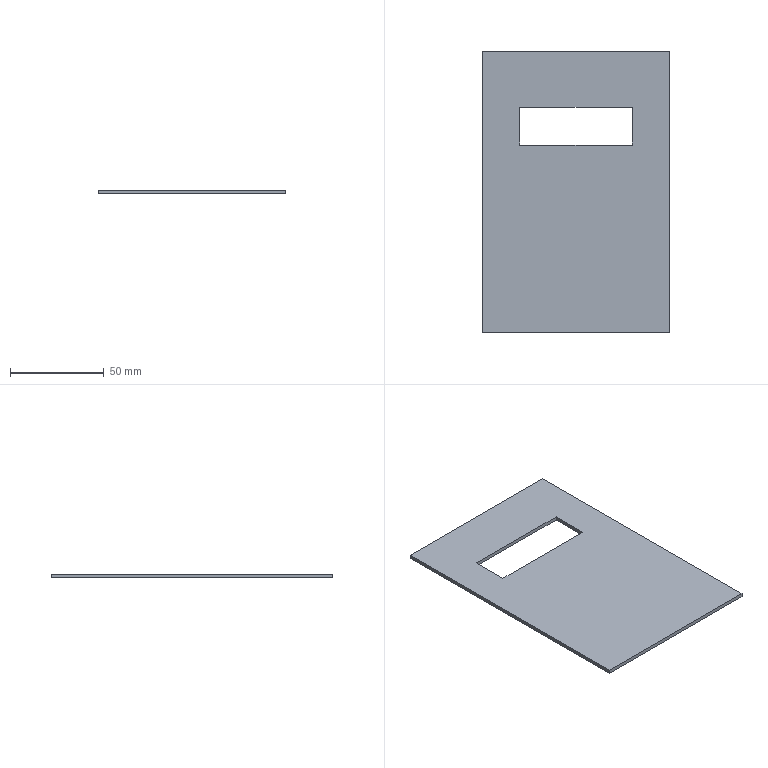Part | NX | 1 solid | 10 faces | box 100 x 150 x 2 mm | volume 27600 mm3 | plane 10
STEP:
#1=CARTESIAN_POINT('',(50.,-75.,0.));
#2=VERTEX_POINT('',#1);
#3=CARTESIAN_POINT('',(50.,75.,0.));
#4=VERTEX_POINT('',#3);
#5=CARTESIAN_POINT('',(50.,75.,0.));
#6=DIRECTION('',(0.,1.,0.));
#7=VECTOR('',#6,1.);
#8=LINE('',#5,#7);
#9=EDGE_CURVE('',#2,#4,#8,.T.);
#10=ORIENTED_EDGE('',*,*,#9,.T.);
#11=CARTESIAN_POINT('',(50.,75.,2.));
#12=VERTEX_POINT('',#11);
#13=CARTESIAN_POINT('',(50.,75.,2.));
#14=DIRECTION('',(0.,0.,-1.));
#15=VECTOR('',#14,1.);
#16=LINE('',#13,#15);
#17=EDGE_CURVE('',#12,#4,#16,.T.);
#18=ORIENTED_EDGE('',*,*,#17,.F.);
#19=CARTESIAN_POINT('',(50.,-75.,2.));
#20=VERTEX_POINT('',#19);
#21=CARTESIAN_POINT('',(50.,75.,2.));
#22=DIRECTION('',(0.,1.,0.));
#23=VECTOR('',#22,1.);
#24=LINE('',#21,#23);
#25=EDGE_CURVE('',#20,#12,#24,.T.);
#26=ORIENTED_EDGE('',*,*,#25,.F.);
#27=CARTESIAN_POINT('',(50.,-75.,2.));
#28=DIRECTION('',(0.,0.,-1.));
#29=VECTOR('',#28,1.);
#30=LINE('',#27,#29);
#31=EDGE_CURVE('',#20,#2,#30,.T.);
#32=ORIENTED_EDGE('',*,*,#31,.T.);
#33=EDGE_LOOP('',(#10,#18,#26,#32));
#34=FACE_OUTER_BOUND('',#33,.T.);
#35=CARTESIAN_POINT('',(50.,75.,2.));
#36=DIRECTION('',(-1.,0.,0.));
#37=DIRECTION('',(0.,-1.,0.));
#38=AXIS2_PLACEMENT_3D('',#35,#36,#37);
#39=PLANE('',#38);
#40=ADVANCED_FACE('',(#34),#39,.F.);
#41=CARTESIAN_POINT('',(-50.,75.,0.));
#42=VERTEX_POINT('',#41);
#43=CARTESIAN_POINT('',(-50.,75.,0.));
#44=DIRECTION('',(-1.,0.,0.));
#45=VECTOR('',#44,1.);
#46=LINE('',#43,#45);
#47=EDGE_CURVE('',#4,#42,#46,.T.);
#48=ORIENTED_EDGE('',*,*,#47,.T.);
#49=CARTESIAN_POINT('',(-50.,75.,2.));
#50=VERTEX_POINT('',#49);
#51=CARTESIAN_POINT('',(-50.,75.,2.));
#52=DIRECTION('',(0.,0.,-1.));
#53=VECTOR('',#52,1.);
#54=LINE('',#51,#53);
#55=EDGE_CURVE('',#50,#42,#54,.T.);
#56=ORIENTED_EDGE('',*,*,#55,.F.);
#57=CARTESIAN_POINT('',(-50.,75.,2.));
#58=DIRECTION('',(-1.,0.,0.));
#59=VECTOR('',#58,1.);
#60=LINE('',#57,#59);
#61=EDGE_CURVE('',#12,#50,#60,.T.);
#62=ORIENTED_EDGE('',*,*,#61,.F.);
#63=ORIENTED_EDGE('',*,*,#17,.T.);
#64=EDGE_LOOP('',(#48,#56,#62,#63));
#65=FACE_OUTER_BOUND('',#64,.T.);
#66=CARTESIAN_POINT('',(-50.,75.,2.));
#67=DIRECTION('',(0.,-1.,0.));
#68=DIRECTION('',(0.,0.,-1.));
#69=AXIS2_PLACEMENT_3D('',#66,#67,#68);
#70=PLANE('',#69);
#71=ADVANCED_FACE('',(#65),#70,.F.);
#72=CARTESIAN_POINT('',(-50.,-75.,0.));
#73=VERTEX_POINT('',#72);
#74=CARTESIAN_POINT('',(-50.,75.,0.));
#75=DIRECTION('',(0.,-1.,0.));
#76=VECTOR('',#75,1.);
#77=LINE('',#74,#76);
#78=EDGE_CURVE('',#42,#73,#77,.T.);
#79=ORIENTED_EDGE('',*,*,#78,.T.);
#80=CARTESIAN_POINT('',(-50.,-75.,2.));
#81=VERTEX_POINT('',#80);
#82=CARTESIAN_POINT('',(-50.,-75.,2.));
#83=DIRECTION('',(0.,0.,-1.));
#84=VECTOR('',#83,1.);
#85=LINE('',#82,#84);
#86=EDGE_CURVE('',#81,#73,#85,.T.);
#87=ORIENTED_EDGE('',*,*,#86,.F.);
#88=CARTESIAN_POINT('',(-50.,75.,2.));
#89=DIRECTION('',(0.,-1.,0.));
#90=VECTOR('',#89,1.);
#91=LINE('',#88,#90);
#92=EDGE_CURVE('',#50,#81,#91,.T.);
#93=ORIENTED_EDGE('',*,*,#92,.F.);
#94=ORIENTED_EDGE('',*,*,#55,.T.);
#95=EDGE_LOOP('',(#79,#87,#93,#94));
#96=FACE_OUTER_BOUND('',#95,.T.);
#97=CARTESIAN_POINT('',(-50.,75.,2.));
#98=DIRECTION('',(1.,0.,0.));
#99=DIRECTION('',(0.,1.,0.));
#100=AXIS2_PLACEMENT_3D('',#97,#98,#99);
#101=PLANE('',#100);
#102=ADVANCED_FACE('',(#96),#101,.F.);
#103=CARTESIAN_POINT('',(-50.,-75.,0.));
#104=DIRECTION('',(1.,0.,0.));
#105=VECTOR('',#104,1.);
#106=LINE('',#103,#105);
#107=EDGE_CURVE('',#73,#2,#106,.T.);
#108=ORIENTED_EDGE('',*,*,#107,.T.);
#109=ORIENTED_EDGE('',*,*,#31,.F.);
#110=CARTESIAN_POINT('',(-50.,-75.,2.));
#111=DIRECTION('',(1.,0.,0.));
#112=VECTOR('',#111,1.);
#113=LINE('',#110,#112);
#114=EDGE_CURVE('',#81,#20,#113,.T.);
#115=ORIENTED_EDGE('',*,*,#114,.F.);
#116=ORIENTED_EDGE('',*,*,#86,.T.);
#117=EDGE_LOOP('',(#108,#109,#115,#116));
#118=FACE_OUTER_BOUND('',#117,.T.);
#119=CARTESIAN_POINT('',(-50.,-75.,2.));
#120=DIRECTION('',(0.,1.,0.));
#121=DIRECTION('',(0.,0.,1.));
#122=AXIS2_PLACEMENT_3D('',#119,#120,#121);
#123=PLANE('',#122);
#124=ADVANCED_FACE('',(#118),#123,.F.);
#125=CARTESIAN_POINT('',(30.,25.,2.));
#126=VERTEX_POINT('',#125);
#127=CARTESIAN_POINT('',(30.,45.,2.));
#128=VERTEX_POINT('',#127);
#129=CARTESIAN_POINT('',(30.,45.,2.));
#130=DIRECTION('',(0.,1.,0.));
#131=VECTOR('',#130,1.);
#132=LINE('',#129,#131);
#133=EDGE_CURVE('',#126,#128,#132,.T.);
#134=ORIENTED_EDGE('',*,*,#133,.F.);
#135=CARTESIAN_POINT('',(-30.,25.,2.));
#136=VERTEX_POINT('',#135);
#137=CARTESIAN_POINT('',(-30.,25.,2.));
#138=DIRECTION('',(1.,0.,0.));
#139=VECTOR('',#138,1.);
#140=LINE('',#137,#139);
#141=EDGE_CURVE('',#136,#126,#140,.T.);
#142=ORIENTED_EDGE('',*,*,#141,.F.);
#143=CARTESIAN_POINT('',(-30.,45.,2.));
#144=VERTEX_POINT('',#143);
#145=CARTESIAN_POINT('',(-30.,45.,2.));
#146=DIRECTION('',(0.,-1.,0.));
#147=VECTOR('',#146,1.);
#148=LINE('',#145,#147);
#149=EDGE_CURVE('',#144,#136,#148,.T.);
#150=ORIENTED_EDGE('',*,*,#149,.F.);
#151=CARTESIAN_POINT('',(-30.,45.,2.));
#152=DIRECTION('',(-1.,0.,0.));
#153=VECTOR('',#152,1.);
#154=LINE('',#151,#153);
#155=EDGE_CURVE('',#128,#144,#154,.T.);
#156=ORIENTED_EDGE('',*,*,#155,.F.);
#157=EDGE_LOOP('',(#134,#142,#150,#156));
#158=FACE_BOUND('',#157,.T.);
#159=ORIENTED_EDGE('',*,*,#25,.T.);
#160=ORIENTED_EDGE('',*,*,#61,.T.);
#161=ORIENTED_EDGE('',*,*,#92,.T.);
#162=ORIENTED_EDGE('',*,*,#114,.T.);
#163=EDGE_LOOP('',(#159,#160,#161,#162));
#164=FACE_BOUND('',#163,.T.);
#165=CARTESIAN_POINT('',(50.,-75.,2.));
#166=DIRECTION('',(0.,0.,1.));
#167=DIRECTION('',(1.,0.,0.));
#168=AXIS2_PLACEMENT_3D('',#165,#166,#167);
#169=PLANE('',#168);
#170=ADVANCED_FACE('',(#158,#164),#169,.T.);
#171=CARTESIAN_POINT('',(-30.,25.,0.));
#172=VERTEX_POINT('',#171);
#173=CARTESIAN_POINT('',(30.,25.,0.));
#174=VERTEX_POINT('',#173);
#175=CARTESIAN_POINT('',(-30.,25.,0.));
#176=DIRECTION('',(1.,0.,0.));
#177=VECTOR('',#176,1.);
#178=LINE('',#175,#177);
#179=EDGE_CURVE('',#172,#174,#178,.T.);
#180=ORIENTED_EDGE('',*,*,#179,.T.);
#181=CARTESIAN_POINT('',(30.,45.,0.));
#182=VERTEX_POINT('',#181);
#183=CARTESIAN_POINT('',(30.,45.,0.));
#184=DIRECTION('',(0.,1.,0.));
#185=VECTOR('',#184,1.);
#186=LINE('',#183,#185);
#187=EDGE_CURVE('',#174,#182,#186,.T.);
#188=ORIENTED_EDGE('',*,*,#187,.T.);
#189=CARTESIAN_POINT('',(-30.,45.,0.));
#190=VERTEX_POINT('',#189);
#191=CARTESIAN_POINT('',(-30.,45.,0.));
#192=DIRECTION('',(-1.,0.,0.));
#193=VECTOR('',#192,1.);
#194=LINE('',#191,#193);
#195=EDGE_CURVE('',#182,#190,#194,.T.);
#196=ORIENTED_EDGE('',*,*,#195,.T.);
#197=CARTESIAN_POINT('',(-30.,45.,0.));
#198=DIRECTION('',(0.,-1.,0.));
#199=VECTOR('',#198,1.);
#200=LINE('',#197,#199);
#201=EDGE_CURVE('',#190,#172,#200,.T.);
#202=ORIENTED_EDGE('',*,*,#201,.T.);
#203=EDGE_LOOP('',(#180,#188,#196,#202));
#204=FACE_BOUND('',#203,.T.);
#205=ORIENTED_EDGE('',*,*,#9,.F.);
#206=ORIENTED_EDGE('',*,*,#107,.F.);
#207=ORIENTED_EDGE('',*,*,#78,.F.);
#208=ORIENTED_EDGE('',*,*,#47,.F.);
#209=EDGE_LOOP('',(#205,#206,#207,#208));
#210=FACE_BOUND('',#209,.T.);
#211=CARTESIAN_POINT('',(50.,-75.,0.));
#212=DIRECTION('',(0.,0.,1.));
#213=DIRECTION('',(1.,0.,0.));
#214=AXIS2_PLACEMENT_3D('',#211,#212,#213);
#215=PLANE('',#214);
#216=ADVANCED_FACE('',(#204,#210),#215,.F.);
#217=ORIENTED_EDGE('',*,*,#133,.T.);
#218=CARTESIAN_POINT('',(30.,45.,0.));
#219=DIRECTION('',(0.,0.,1.));
#220=VECTOR('',#219,1.);
#221=LINE('',#218,#220);
#222=EDGE_CURVE('',#182,#128,#221,.T.);
#223=ORIENTED_EDGE('',*,*,#222,.F.);
#224=ORIENTED_EDGE('',*,*,#187,.F.);
#225=CARTESIAN_POINT('',(30.,25.,0.));
#226=DIRECTION('',(0.,0.,1.));
#227=VECTOR('',#226,1.);
#228=LINE('',#225,#227);
#229=EDGE_CURVE('',#174,#126,#228,.T.);
#230=ORIENTED_EDGE('',*,*,#229,.T.);
#231=EDGE_LOOP('',(#217,#223,#224,#230));
#232=FACE_OUTER_BOUND('',#231,.T.);
#233=CARTESIAN_POINT('',(30.,45.,0.));
#234=DIRECTION('',(1.,0.,0.));
#235=DIRECTION('',(0.,1.,0.));
#236=AXIS2_PLACEMENT_3D('',#233,#234,#235);
#237=PLANE('',#236);
#238=ADVANCED_FACE('',(#232),#237,.F.);
#239=ORIENTED_EDGE('',*,*,#141,.T.);
#240=ORIENTED_EDGE('',*,*,#229,.F.);
#241=ORIENTED_EDGE('',*,*,#179,.F.);
#242=CARTESIAN_POINT('',(-30.,25.,0.));
#243=DIRECTION('',(0.,0.,1.));
#244=VECTOR('',#243,1.);
#245=LINE('',#242,#244);
#246=EDGE_CURVE('',#172,#136,#245,.T.);
#247=ORIENTED_EDGE('',*,*,#246,.T.);
#248=EDGE_LOOP('',(#239,#240,#241,#247));
#249=FACE_OUTER_BOUND('',#248,.T.);
#250=CARTESIAN_POINT('',(-30.,25.,0.));
#251=DIRECTION('',(0.,-1.,0.));
#252=DIRECTION('',(0.,0.,-1.));
#253=AXIS2_PLACEMENT_3D('',#250,#251,#252);
#254=PLANE('',#253);
#255=ADVANCED_FACE('',(#249),#254,.F.);
#256=ORIENTED_EDGE('',*,*,#149,.T.);
#257=ORIENTED_EDGE('',*,*,#246,.F.);
#258=ORIENTED_EDGE('',*,*,#201,.F.);
#259=CARTESIAN_POINT('',(-30.,45.,0.));
#260=DIRECTION('',(0.,0.,1.));
#261=VECTOR('',#260,1.);
#262=LINE('',#259,#261);
#263=EDGE_CURVE('',#190,#144,#262,.T.);
#264=ORIENTED_EDGE('',*,*,#263,.T.);
#265=EDGE_LOOP('',(#256,#257,#258,#264));
#266=FACE_OUTER_BOUND('',#265,.T.);
#267=CARTESIAN_POINT('',(-30.,45.,0.));
#268=DIRECTION('',(-1.,0.,0.));
#269=DIRECTION('',(0.,-1.,0.));
#270=AXIS2_PLACEMENT_3D('',#267,#268,#269);
#271=PLANE('',#270);
#272=ADVANCED_FACE('',(#266),#271,.F.);
#273=ORIENTED_EDGE('',*,*,#155,.T.);
#274=ORIENTED_EDGE('',*,*,#263,.F.);
#275=ORIENTED_EDGE('',*,*,#195,.F.);
#276=ORIENTED_EDGE('',*,*,#222,.T.);
#277=EDGE_LOOP('',(#273,#274,#275,#276));
#278=FACE_OUTER_BOUND('',#277,.T.);
#279=CARTESIAN_POINT('',(-30.,45.,0.));
#280=DIRECTION('',(0.,1.,0.));
#281=DIRECTION('',(0.,0.,1.));
#282=AXIS2_PLACEMENT_3D('',#279,#280,#281);
#283=PLANE('',#282);
#284=ADVANCED_FACE('',(#278),#283,.F.);
#285=CLOSED_SHELL('',(#40,#71,#102,#124,#170,#216,#238,#255,#272,#284));
#286=MANIFOLD_SOLID_BREP('',#285);
#287=(LENGTH_UNIT()NAMED_UNIT(*)SI_UNIT(.MILLI.,.METRE.));
#288=UNCERTAINTY_MEASURE_WITH_UNIT(LENGTH_MEASURE(0.00002),#287,'','');
#289=(NAMED_UNIT(*)PLANE_ANGLE_UNIT()SI_UNIT($,.RADIAN.));
#290=PLANE_ANGLE_MEASURE_WITH_UNIT(PLANE_ANGLE_MEASURE(0.01745),#289);
#291=DIMENSIONAL_EXPONENTS(0.,0.,0.,0.,0.,0.,0.);
#292=(CONVERSION_BASED_UNIT('DEGREE',#290)NAMED_UNIT(#291)PLANE_ANGLE_UNIT());
#293=(NAMED_UNIT(*)SI_UNIT($,.STERADIAN.)SOLID_ANGLE_UNIT());
#294=(GEOMETRIC_REPRESENTATION_CONTEXT(3)GLOBAL_UNCERTAINTY_ASSIGNED_CONTEXT((#288))GLOBAL_UNIT_ASSIGNED_CONTEXT((#287,#292,#293))REPRESENTATION_CONTEXT('',''));
#295=ADVANCED_BREP_SHAPE_REPRESENTATION('',(#286),#294);